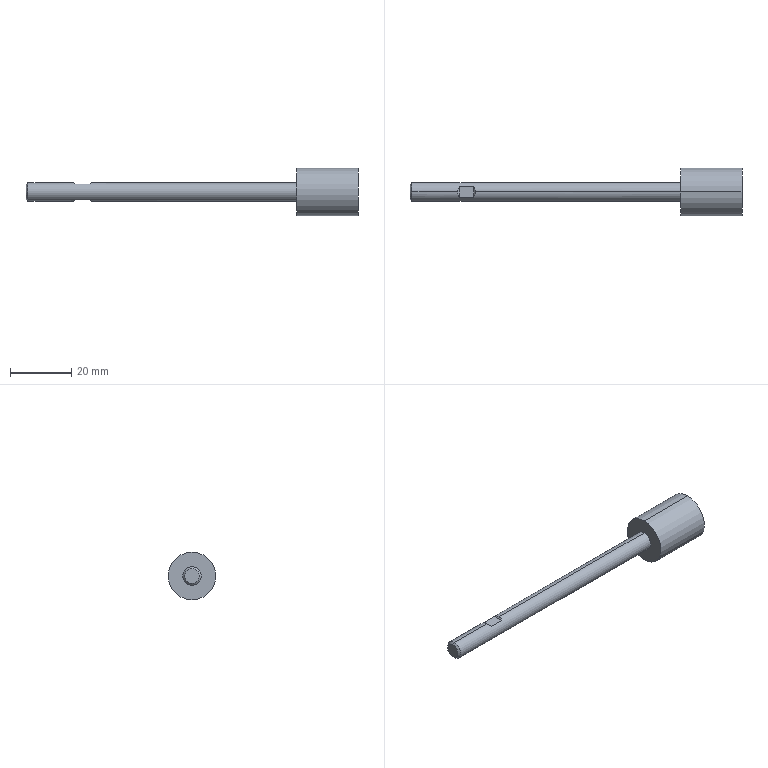Part | SolidWorks | features BaseBody 1 | 1 solid | 15 faces | box 108 x 15.5 x 15.5 mm | volume 6247 mm3 | plane 9 | cylinder 4 | cone 2 | commonest cylinder face diameters 6 x2 15.5 x2
STEP:
#1=CARTESIAN_POINT('',(88.,0.,3.));
#2=VERTEX_POINT('',#1);
#3=CARTESIAN_POINT('',(88.,0.,-3.));
#4=VERTEX_POINT('',#3);
#5=CARTESIAN_POINT('',(88.,0.,0.));
#6=DIRECTION('',(1.,0.,0.));
#7=DIRECTION('',(0.,0.,-1.));
#8=AXIS2_PLACEMENT_3D('',#5,#6,#7);
#9=CIRCLE('',#8,3.);
#10=EDGE_CURVE('',#2,#4,#9,.T.);
#11=ORIENTED_EDGE('',*,*,#10,.F.);
#12=CARTESIAN_POINT('',(21.3,0.,3.));
#13=VERTEX_POINT('',#12);
#14=CARTESIAN_POINT('',(108.,0.,3.));
#15=DIRECTION('',(-1.,0.,0.));
#16=VECTOR('',#15,1000.);
#17=LINE('',#14,#16);
#18=EDGE_CURVE('',#2,#13,#17,.T.);
#19=ORIENTED_EDGE('',*,*,#18,.T.);
#20=CARTESIAN_POINT('',(20.8,-1.658,2.5));
#21=VERTEX_POINT('',#20);
#22=CARTESIAN_POINT('',(20.8,-1.658,2.5));
#23=CARTESIAN_POINT('',(21.128,-1.163,2.828));
#24=CARTESIAN_POINT('',(21.3,-0.5942,3.));
#25=CARTESIAN_POINT('',(21.3,0.,3.));
#26=(BOUNDED_CURVE()B_SPLINE_CURVE(3,(#22,#23,#24,#25),.UNSPECIFIED.,.F.,.F.)B_SPLINE_CURVE_WITH_KNOTS((4,4),(5.697,6.283),.UNSPECIFIED.)CURVE()GEOMETRIC_REPRESENTATION_ITEM()RATIONAL_B_SPLINE_CURVE((1.,0.9716,0.9716,1.))REPRESENTATION_ITEM(''));
#27=EDGE_CURVE('',#21,#13,#26,.T.);
#28=ORIENTED_EDGE('',*,*,#27,.F.);
#29=CARTESIAN_POINT('',(16.,-1.658,2.5));
#30=VERTEX_POINT('',#29);
#31=CARTESIAN_POINT('',(108.,-1.658,2.5));
#32=DIRECTION('',(1.,0.,0.));
#33=VECTOR('',#32,1000.);
#34=LINE('',#31,#33);
#35=EDGE_CURVE('',#30,#21,#34,.T.);
#36=ORIENTED_EDGE('',*,*,#35,.F.);
#37=CARTESIAN_POINT('',(15.5,0.,3.));
#38=VERTEX_POINT('',#37);
#39=CARTESIAN_POINT('',(15.5,0.,3.));
#40=CARTESIAN_POINT('',(15.5,-0.5942,3.));
#41=CARTESIAN_POINT('',(15.672,-1.163,2.828));
#42=CARTESIAN_POINT('',(16.,-1.658,2.5));
#43=(BOUNDED_CURVE()B_SPLINE_CURVE(3,(#39,#40,#41,#42),.UNSPECIFIED.,.F.,.F.)B_SPLINE_CURVE_WITH_KNOTS((4,4),(3.142,3.727),.UNSPECIFIED.)CURVE()GEOMETRIC_REPRESENTATION_ITEM()RATIONAL_B_SPLINE_CURVE((1.,0.9716,0.9716,1.))REPRESENTATION_ITEM(''));
#44=EDGE_CURVE('',#38,#30,#43,.T.);
#45=ORIENTED_EDGE('',*,*,#44,.F.);
#46=CARTESIAN_POINT('',(0.6135,0.,3.));
#47=VERTEX_POINT('',#46);
#48=CARTESIAN_POINT('',(108.,0.,3.));
#49=DIRECTION('',(-1.,0.,0.));
#50=VECTOR('',#49,1000.);
#51=LINE('',#48,#50);
#52=EDGE_CURVE('',#38,#47,#51,.T.);
#53=ORIENTED_EDGE('',*,*,#52,.T.);
#54=CARTESIAN_POINT('',(0.6135,0.,-3.));
#55=VERTEX_POINT('',#54);
#56=CARTESIAN_POINT('',(0.6135,0.,0.));
#57=DIRECTION('',(1.,0.,0.));
#58=DIRECTION('',(0.,0.,-1.));
#59=AXIS2_PLACEMENT_3D('',#56,#57,#58);
#60=CIRCLE('',#59,3.);
#61=EDGE_CURVE('',#47,#55,#60,.T.);
#62=ORIENTED_EDGE('',*,*,#61,.T.);
#63=CARTESIAN_POINT('',(15.5,0.,-3.));
#64=VERTEX_POINT('',#63);
#65=CARTESIAN_POINT('',(108.,0.,-3.));
#66=DIRECTION('',(-1.,0.,0.));
#67=VECTOR('',#66,1000.);
#68=LINE('',#65,#67);
#69=EDGE_CURVE('',#64,#55,#68,.T.);
#70=ORIENTED_EDGE('',*,*,#69,.F.);
#71=CARTESIAN_POINT('',(16.,-1.658,-2.5));
#72=VERTEX_POINT('',#71);
#73=CARTESIAN_POINT('',(16.,-1.658,-2.5));
#74=CARTESIAN_POINT('',(15.672,-1.163,-2.828));
#75=CARTESIAN_POINT('',(15.5,-0.5942,-3.));
#76=CARTESIAN_POINT('',(15.5,0.,-3.));
#77=(BOUNDED_CURVE()B_SPLINE_CURVE(3,(#73,#74,#75,#76),.UNSPECIFIED.,.F.,.F.)B_SPLINE_CURVE_WITH_KNOTS((4,4),(2.556,3.142),.UNSPECIFIED.)CURVE()GEOMETRIC_REPRESENTATION_ITEM()RATIONAL_B_SPLINE_CURVE((1.,0.9716,0.9716,1.))REPRESENTATION_ITEM(''));
#78=EDGE_CURVE('',#72,#64,#77,.T.);
#79=ORIENTED_EDGE('',*,*,#78,.F.);
#80=CARTESIAN_POINT('',(20.8,-1.658,-2.5));
#81=VERTEX_POINT('',#80);
#82=CARTESIAN_POINT('',(108.,-1.658,-2.5));
#83=DIRECTION('',(-1.,0.,0.));
#84=VECTOR('',#83,1000.);
#85=LINE('',#82,#84);
#86=EDGE_CURVE('',#81,#72,#85,.T.);
#87=ORIENTED_EDGE('',*,*,#86,.F.);
#88=CARTESIAN_POINT('',(21.3,0.,-3.));
#89=VERTEX_POINT('',#88);
#90=CARTESIAN_POINT('',(21.3,0.,-3.));
#91=CARTESIAN_POINT('',(21.3,-0.5942,-3.));
#92=CARTESIAN_POINT('',(21.128,-1.163,-2.828));
#93=CARTESIAN_POINT('',(20.8,-1.658,-2.5));
#94=(BOUNDED_CURVE()B_SPLINE_CURVE(3,(#90,#91,#92,#93),.UNSPECIFIED.,.F.,.T.)B_SPLINE_CURVE_WITH_KNOTS((4,4),(0.,0.5857),.UNSPECIFIED.)CURVE()GEOMETRIC_REPRESENTATION_ITEM()RATIONAL_B_SPLINE_CURVE((1.,0.9716,0.9716,1.))REPRESENTATION_ITEM(''));
#95=EDGE_CURVE('',#89,#81,#94,.T.);
#96=ORIENTED_EDGE('',*,*,#95,.F.);
#97=CARTESIAN_POINT('',(108.,0.,-3.));
#98=DIRECTION('',(-1.,0.,0.));
#99=VECTOR('',#98,1000.);
#100=LINE('',#97,#99);
#101=EDGE_CURVE('',#4,#89,#100,.T.);
#102=ORIENTED_EDGE('',*,*,#101,.F.);
#103=EDGE_LOOP('',(#11,#19,#28,#36,#45,#53,#62,#70,#79,#87,#96,#102));
#104=FACE_OUTER_BOUND('',#103,.T.);
#105=CARTESIAN_POINT('',(108.,0.,0.));
#106=DIRECTION('',(-1.,0.,0.));
#107=DIRECTION('',(0.,0.,-1.));
#108=AXIS2_PLACEMENT_3D('',#105,#106,#107);
#109=CYLINDRICAL_SURFACE('',#108,3.);
#110=ADVANCED_FACE('',(#104),#109,.T.);
#111=CARTESIAN_POINT('',(0.,0.,-2.387));
#112=VERTEX_POINT('',#111);
#113=CARTESIAN_POINT('',(0.,0.,2.387));
#114=VERTEX_POINT('',#113);
#115=CARTESIAN_POINT('',(0.,0.,0.));
#116=DIRECTION('',(1.,0.,0.));
#117=DIRECTION('',(0.,0.,-1.));
#118=AXIS2_PLACEMENT_3D('',#115,#116,#117);
#119=CIRCLE('',#118,2.387);
#120=EDGE_CURVE('',#112,#114,#119,.T.);
#121=ORIENTED_EDGE('',*,*,#120,.T.);
#122=CARTESIAN_POINT('',(0.,0.,2.387));
#123=DIRECTION('',(0.7071,0.,0.7071));
#124=VECTOR('',#123,1000.);
#125=LINE('',#122,#124);
#126=EDGE_CURVE('',#114,#47,#125,.T.);
#127=ORIENTED_EDGE('',*,*,#126,.T.);
#128=CARTESIAN_POINT('',(0.6135,0.,0.));
#129=DIRECTION('',(1.,0.,0.));
#130=DIRECTION('',(0.,0.,-1.));
#131=AXIS2_PLACEMENT_3D('',#128,#129,#130);
#132=CIRCLE('',#131,3.);
#133=EDGE_CURVE('',#55,#47,#132,.T.);
#134=ORIENTED_EDGE('',*,*,#133,.F.);
#135=CARTESIAN_POINT('',(0.,0.,-2.387));
#136=DIRECTION('',(0.7071,0.,-0.7071));
#137=VECTOR('',#136,1000.);
#138=LINE('',#135,#137);
#139=EDGE_CURVE('',#112,#55,#138,.T.);
#140=ORIENTED_EDGE('',*,*,#139,.F.);
#141=EDGE_LOOP('',(#121,#127,#134,#140));
#142=FACE_OUTER_BOUND('',#141,.T.);
#143=CARTESIAN_POINT('',(0.,0.,0.));
#144=DIRECTION('',(1.,0.,0.));
#145=DIRECTION('',(0.,0.,-1.));
#146=AXIS2_PLACEMENT_3D('',#143,#144,#145);
#147=CONICAL_SURFACE('',#146,2.387,0.7854);
#148=ADVANCED_FACE('',(#142),#147,.T.);
#149=CARTESIAN_POINT('',(108.,0.,7.75));
#150=VERTEX_POINT('',#149);
#151=CARTESIAN_POINT('',(108.,0.,-7.75));
#152=VERTEX_POINT('',#151);
#153=CARTESIAN_POINT('',(108.,0.,0.));
#154=DIRECTION('',(1.,0.,0.));
#155=DIRECTION('',(0.,0.,-1.));
#156=AXIS2_PLACEMENT_3D('',#153,#154,#155);
#157=CIRCLE('',#156,7.75);
#158=EDGE_CURVE('',#150,#152,#157,.T.);
#159=ORIENTED_EDGE('',*,*,#158,.F.);
#160=CARTESIAN_POINT('',(88.,0.,7.75));
#161=VERTEX_POINT('',#160);
#162=CARTESIAN_POINT('',(108.,0.,7.75));
#163=DIRECTION('',(-1.,0.,0.));
#164=VECTOR('',#163,1000.);
#165=LINE('',#162,#164);
#166=EDGE_CURVE('',#150,#161,#165,.T.);
#167=ORIENTED_EDGE('',*,*,#166,.T.);
#168=CARTESIAN_POINT('',(88.,0.,-7.75));
#169=VERTEX_POINT('',#168);
#170=CARTESIAN_POINT('',(88.,0.,0.));
#171=DIRECTION('',(1.,0.,0.));
#172=DIRECTION('',(0.,0.,-1.));
#173=AXIS2_PLACEMENT_3D('',#170,#171,#172);
#174=CIRCLE('',#173,7.75);
#175=EDGE_CURVE('',#161,#169,#174,.T.);
#176=ORIENTED_EDGE('',*,*,#175,.T.);
#177=CARTESIAN_POINT('',(108.,0.,-7.75));
#178=DIRECTION('',(-1.,0.,0.));
#179=VECTOR('',#178,1000.);
#180=LINE('',#177,#179);
#181=EDGE_CURVE('',#152,#169,#180,.T.);
#182=ORIENTED_EDGE('',*,*,#181,.F.);
#183=EDGE_LOOP('',(#159,#167,#176,#182));
#184=FACE_OUTER_BOUND('',#183,.T.);
#185=CARTESIAN_POINT('',(108.,0.,0.));
#186=DIRECTION('',(-1.,0.,0.));
#187=DIRECTION('',(0.,0.,-1.));
#188=AXIS2_PLACEMENT_3D('',#185,#186,#187);
#189=CYLINDRICAL_SURFACE('',#188,7.75);
#190=ADVANCED_FACE('',(#184),#189,.T.);
#191=ORIENTED_EDGE('',*,*,#166,.F.);
#192=CARTESIAN_POINT('',(108.,0.,0.));
#193=DIRECTION('',(1.,0.,0.));
#194=DIRECTION('',(0.,0.,-1.));
#195=AXIS2_PLACEMENT_3D('',#192,#193,#194);
#196=CIRCLE('',#195,7.75);
#197=EDGE_CURVE('',#152,#150,#196,.T.);
#198=ORIENTED_EDGE('',*,*,#197,.F.);
#199=ORIENTED_EDGE('',*,*,#181,.T.);
#200=CARTESIAN_POINT('',(88.,0.,0.));
#201=DIRECTION('',(1.,0.,0.));
#202=DIRECTION('',(0.,0.,-1.));
#203=AXIS2_PLACEMENT_3D('',#200,#201,#202);
#204=CIRCLE('',#203,7.75);
#205=EDGE_CURVE('',#169,#161,#204,.T.);
#206=ORIENTED_EDGE('',*,*,#205,.T.);
#207=EDGE_LOOP('',(#191,#198,#199,#206));
#208=FACE_OUTER_BOUND('',#207,.T.);
#209=CARTESIAN_POINT('',(108.,0.,0.));
#210=DIRECTION('',(-1.,0.,0.));
#211=DIRECTION('',(0.,0.,-1.));
#212=AXIS2_PLACEMENT_3D('',#209,#210,#211);
#213=CYLINDRICAL_SURFACE('',#212,7.75);
#214=ADVANCED_FACE('',(#208),#213,.T.);
#215=ORIENTED_EDGE('',*,*,#197,.T.);
#216=ORIENTED_EDGE('',*,*,#158,.T.);
#217=EDGE_LOOP('',(#215,#216));
#218=FACE_OUTER_BOUND('',#217,.T.);
#219=CARTESIAN_POINT('',(108.,7.75,0.));
#220=DIRECTION('',(-1.,0.,0.));
#221=DIRECTION('',(0.,0.,1.));
#222=AXIS2_PLACEMENT_3D('',#219,#220,#221);
#223=PLANE('',#222);
#224=ADVANCED_FACE('',(#218),#223,.F.);
#225=CARTESIAN_POINT('',(20.8,1.658,-2.5));
#226=VERTEX_POINT('',#225);
#227=CARTESIAN_POINT('',(20.8,1.658,-2.5));
#228=CARTESIAN_POINT('',(21.128,1.163,-2.828));
#229=CARTESIAN_POINT('',(21.3,0.5942,-3.));
#230=CARTESIAN_POINT('',(21.3,0.,-3.));
#231=(BOUNDED_CURVE()B_SPLINE_CURVE(3,(#227,#228,#229,#230),.UNSPECIFIED.,.F.,.F.)B_SPLINE_CURVE_WITH_KNOTS((4,4),(5.697,6.283),.UNSPECIFIED.)CURVE()GEOMETRIC_REPRESENTATION_ITEM()RATIONAL_B_SPLINE_CURVE((1.,0.9716,0.9716,1.))REPRESENTATION_ITEM(''));
#232=EDGE_CURVE('',#226,#89,#231,.T.);
#233=ORIENTED_EDGE('',*,*,#232,.T.);
#234=ORIENTED_EDGE('',*,*,#95,.T.);
#235=CARTESIAN_POINT('',(20.8,2.5,-2.5));
#236=DIRECTION('',(0.,-1.,0.));
#237=VECTOR('',#236,1000.);
#238=LINE('',#235,#237);
#239=EDGE_CURVE('',#226,#81,#238,.T.);
#240=ORIENTED_EDGE('',*,*,#239,.F.);
#241=EDGE_LOOP('',(#233,#234,#240));
#242=FACE_OUTER_BOUND('',#241,.T.);
#243=CARTESIAN_POINT('',(20.8,2.5,-2.5));
#244=DIRECTION('',(-0.7071,0.,-0.7071));
#245=DIRECTION('',(-0.7071,0.,0.7071));
#246=AXIS2_PLACEMENT_3D('',#243,#244,#245);
#247=PLANE('',#246);
#248=ADVANCED_FACE('',(#242),#247,.T.);
#249=CARTESIAN_POINT('',(16.,1.658,-2.5));
#250=VERTEX_POINT('',#249);
#251=CARTESIAN_POINT('',(108.,1.658,-2.5));
#252=DIRECTION('',(1.,0.,0.));
#253=VECTOR('',#252,1000.);
#254=LINE('',#251,#253);
#255=EDGE_CURVE('',#250,#226,#254,.T.);
#256=ORIENTED_EDGE('',*,*,#255,.T.);
#257=ORIENTED_EDGE('',*,*,#239,.T.);
#258=ORIENTED_EDGE('',*,*,#86,.T.);
#259=CARTESIAN_POINT('',(16.,2.5,-2.5));
#260=DIRECTION('',(0.,-1.,0.));
#261=VECTOR('',#260,1000.);
#262=LINE('',#259,#261);
#263=EDGE_CURVE('',#250,#72,#262,.T.);
#264=ORIENTED_EDGE('',*,*,#263,.F.);
#265=EDGE_LOOP('',(#256,#257,#258,#264));
#266=FACE_OUTER_BOUND('',#265,.T.);
#267=CARTESIAN_POINT('',(16.,2.5,-2.5));
#268=DIRECTION('',(0.,0.,-1.));
#269=DIRECTION('',(0.,-1.,0.));
#270=AXIS2_PLACEMENT_3D('',#267,#268,#269);
#271=PLANE('',#270);
#272=ADVANCED_FACE('',(#266),#271,.T.);
#273=ORIENTED_EDGE('',*,*,#27,.T.);
#274=CARTESIAN_POINT('',(20.8,1.658,2.5));
#275=VERTEX_POINT('',#274);
#276=CARTESIAN_POINT('',(21.3,0.,3.));
#277=CARTESIAN_POINT('',(21.3,0.5942,3.));
#278=CARTESIAN_POINT('',(21.128,1.163,2.828));
#279=CARTESIAN_POINT('',(20.8,1.658,2.5));
#280=(BOUNDED_CURVE()B_SPLINE_CURVE(3,(#276,#277,#278,#279),.UNSPECIFIED.,.F.,.F.)B_SPLINE_CURVE_WITH_KNOTS((4,4),(0.,0.5857),.UNSPECIFIED.)CURVE()GEOMETRIC_REPRESENTATION_ITEM()RATIONAL_B_SPLINE_CURVE((1.,0.9716,0.9716,1.))REPRESENTATION_ITEM(''));
#281=EDGE_CURVE('',#13,#275,#280,.T.);
#282=ORIENTED_EDGE('',*,*,#281,.T.);
#283=CARTESIAN_POINT('',(20.8,2.5,2.5));
#284=DIRECTION('',(0.,-1.,0.));
#285=VECTOR('',#284,1000.);
#286=LINE('',#283,#285);
#287=EDGE_CURVE('',#275,#21,#286,.T.);
#288=ORIENTED_EDGE('',*,*,#287,.T.);
#289=EDGE_LOOP('',(#273,#282,#288));
#290=FACE_OUTER_BOUND('',#289,.T.);
#291=CARTESIAN_POINT('',(30.3,2.5,12.));
#292=DIRECTION('',(-0.7071,0.,0.7071));
#293=DIRECTION('',(0.,1.,0.));
#294=AXIS2_PLACEMENT_3D('',#291,#292,#293);
#295=PLANE('',#294);
#296=ADVANCED_FACE('',(#290),#295,.T.);
#297=ORIENTED_EDGE('',*,*,#78,.T.);
#298=CARTESIAN_POINT('',(15.5,0.,-3.));
#299=CARTESIAN_POINT('',(15.5,0.5942,-3.));
#300=CARTESIAN_POINT('',(15.672,1.163,-2.828));
#301=CARTESIAN_POINT('',(16.,1.658,-2.5));
#302=(BOUNDED_CURVE()B_SPLINE_CURVE(3,(#298,#299,#300,#301),.UNSPECIFIED.,.F.,.F.)B_SPLINE_CURVE_WITH_KNOTS((4,4),(3.142,3.727),.UNSPECIFIED.)CURVE()GEOMETRIC_REPRESENTATION_ITEM()RATIONAL_B_SPLINE_CURVE((1.,0.9716,0.9716,1.))REPRESENTATION_ITEM(''));
#303=EDGE_CURVE('',#64,#250,#302,.T.);
#304=ORIENTED_EDGE('',*,*,#303,.T.);
#305=ORIENTED_EDGE('',*,*,#263,.T.);
#306=EDGE_LOOP('',(#297,#304,#305));
#307=FACE_OUTER_BOUND('',#306,.T.);
#308=CARTESIAN_POINT('',(14.4,2.5,-4.1));
#309=DIRECTION('',(0.7071,0.,-0.7071));
#310=DIRECTION('',(0.,-1.,0.));
#311=AXIS2_PLACEMENT_3D('',#308,#309,#310);
#312=PLANE('',#311);
#313=ADVANCED_FACE('',(#307),#312,.T.);
#314=CARTESIAN_POINT('',(88.,0.,0.));
#315=DIRECTION('',(1.,0.,0.));
#316=DIRECTION('',(0.,0.,-1.));
#317=AXIS2_PLACEMENT_3D('',#314,#315,#316);
#318=CIRCLE('',#317,3.);
#319=EDGE_CURVE('',#4,#2,#318,.T.);
#320=ORIENTED_EDGE('',*,*,#319,.T.);
#321=ORIENTED_EDGE('',*,*,#10,.T.);
#322=EDGE_LOOP('',(#320,#321));
#323=FACE_BOUND('',#322,.T.);
#324=ORIENTED_EDGE('',*,*,#205,.F.);
#325=ORIENTED_EDGE('',*,*,#175,.F.);
#326=EDGE_LOOP('',(#324,#325));
#327=FACE_OUTER_BOUND('',#326,.T.);
#328=CARTESIAN_POINT('',(88.,3.,0.));
#329=DIRECTION('',(1.,0.,0.));
#330=DIRECTION('',(0.,1.,0.));
#331=AXIS2_PLACEMENT_3D('',#328,#329,#330);
#332=PLANE('',#331);
#333=ADVANCED_FACE('',(#323,#327),#332,.F.);
#334=ORIENTED_EDGE('',*,*,#126,.F.);
#335=CARTESIAN_POINT('',(0.,0.,0.));
#336=DIRECTION('',(1.,0.,0.));
#337=DIRECTION('',(0.,0.,-1.));
#338=AXIS2_PLACEMENT_3D('',#335,#336,#337);
#339=CIRCLE('',#338,2.387);
#340=EDGE_CURVE('',#114,#112,#339,.T.);
#341=ORIENTED_EDGE('',*,*,#340,.T.);
#342=ORIENTED_EDGE('',*,*,#139,.T.);
#343=ORIENTED_EDGE('',*,*,#61,.F.);
#344=EDGE_LOOP('',(#334,#341,#342,#343));
#345=FACE_OUTER_BOUND('',#344,.T.);
#346=CARTESIAN_POINT('',(0.,0.,0.));
#347=DIRECTION('',(1.,0.,0.));
#348=DIRECTION('',(0.,0.,-1.));
#349=AXIS2_PLACEMENT_3D('',#346,#347,#348);
#350=CONICAL_SURFACE('',#349,2.387,0.7854);
#351=ADVANCED_FACE('',(#345),#350,.T.);
#352=ORIENTED_EDGE('',*,*,#120,.F.);
#353=ORIENTED_EDGE('',*,*,#340,.F.);
#354=EDGE_LOOP('',(#352,#353));
#355=FACE_OUTER_BOUND('',#354,.T.);
#356=CARTESIAN_POINT('',(0.,0.,0.));
#357=DIRECTION('',(1.,0.,0.));
#358=DIRECTION('',(0.,1.,0.));
#359=AXIS2_PLACEMENT_3D('',#356,#357,#358);
#360=PLANE('',#359);
#361=ADVANCED_FACE('',(#355),#360,.F.);
#362=ORIENTED_EDGE('',*,*,#18,.F.);
#363=ORIENTED_EDGE('',*,*,#319,.F.);
#364=ORIENTED_EDGE('',*,*,#101,.T.);
#365=ORIENTED_EDGE('',*,*,#232,.F.);
#366=ORIENTED_EDGE('',*,*,#255,.F.);
#367=ORIENTED_EDGE('',*,*,#303,.F.);
#368=ORIENTED_EDGE('',*,*,#69,.T.);
#369=ORIENTED_EDGE('',*,*,#133,.T.);
#370=ORIENTED_EDGE('',*,*,#52,.F.);
#371=CARTESIAN_POINT('',(16.,1.658,2.5));
#372=VERTEX_POINT('',#371);
#373=CARTESIAN_POINT('',(16.,1.658,2.5));
#374=CARTESIAN_POINT('',(15.672,1.163,2.828));
#375=CARTESIAN_POINT('',(15.5,0.5942,3.));
#376=CARTESIAN_POINT('',(15.5,0.,3.));
#377=(BOUNDED_CURVE()B_SPLINE_CURVE(3,(#373,#374,#375,#376),.UNSPECIFIED.,.F.,.F.)B_SPLINE_CURVE_WITH_KNOTS((4,4),(2.556,3.142),.UNSPECIFIED.)CURVE()GEOMETRIC_REPRESENTATION_ITEM()RATIONAL_B_SPLINE_CURVE((1.,0.9716,0.9716,1.))REPRESENTATION_ITEM(''));
#378=EDGE_CURVE('',#372,#38,#377,.T.);
#379=ORIENTED_EDGE('',*,*,#378,.F.);
#380=CARTESIAN_POINT('',(108.,1.658,2.5));
#381=DIRECTION('',(-1.,0.,0.));
#382=VECTOR('',#381,1000.);
#383=LINE('',#380,#382);
#384=EDGE_CURVE('',#275,#372,#383,.T.);
#385=ORIENTED_EDGE('',*,*,#384,.F.);
#386=ORIENTED_EDGE('',*,*,#281,.F.);
#387=EDGE_LOOP('',(#362,#363,#364,#365,#366,#367,#368,#369,#370,#379,#385,#386));
#388=FACE_OUTER_BOUND('',#387,.T.);
#389=CARTESIAN_POINT('',(108.,0.,0.));
#390=DIRECTION('',(-1.,0.,0.));
#391=DIRECTION('',(0.,0.,-1.));
#392=AXIS2_PLACEMENT_3D('',#389,#390,#391);
#393=CYLINDRICAL_SURFACE('',#392,3.);
#394=ADVANCED_FACE('',(#388),#393,.T.);
#395=ORIENTED_EDGE('',*,*,#35,.T.);
#396=ORIENTED_EDGE('',*,*,#287,.F.);
#397=ORIENTED_EDGE('',*,*,#384,.T.);
#398=CARTESIAN_POINT('',(16.,2.5,2.5));
#399=DIRECTION('',(0.,-1.,0.));
#400=VECTOR('',#399,1000.);
#401=LINE('',#398,#400);
#402=EDGE_CURVE('',#372,#30,#401,.T.);
#403=ORIENTED_EDGE('',*,*,#402,.T.);
#404=EDGE_LOOP('',(#395,#396,#397,#403));
#405=FACE_OUTER_BOUND('',#404,.T.);
#406=CARTESIAN_POINT('',(20.8,2.5,2.5));
#407=DIRECTION('',(0.,0.,1.));
#408=DIRECTION('',(1.,0.,0.));
#409=AXIS2_PLACEMENT_3D('',#406,#407,#408);
#410=PLANE('',#409);
#411=ADVANCED_FACE('',(#405),#410,.T.);
#412=ORIENTED_EDGE('',*,*,#378,.T.);
#413=ORIENTED_EDGE('',*,*,#44,.T.);
#414=ORIENTED_EDGE('',*,*,#402,.F.);
#415=EDGE_LOOP('',(#412,#413,#414));
#416=FACE_OUTER_BOUND('',#415,.T.);
#417=CARTESIAN_POINT('',(16.,2.5,2.5));
#418=DIRECTION('',(0.7071,0.,0.7071));
#419=DIRECTION('',(0.,-1.,0.));
#420=AXIS2_PLACEMENT_3D('',#417,#418,#419);
#421=PLANE('',#420);
#422=ADVANCED_FACE('',(#416),#421,.T.);
#423=CLOSED_SHELL('',(#110,#148,#190,#214,#224,#248,#272,#296,#313,#333,#351,#361,#394,#411,#422));
#424=MANIFOLD_SOLID_BREP('',#423);
#425=CARTESIAN_POINT('',(0.,0.,0.));
#426=DIRECTION('',(0.,0.,1.));
#427=DIRECTION('',(1.,0.,0.));
#428=AXIS2_PLACEMENT_3D('',#425,#426,#427);
#429=(LENGTH_UNIT()NAMED_UNIT(*)SI_UNIT(.MILLI.,.METRE.));
#430=UNCERTAINTY_MEASURE_WITH_UNIT(LENGTH_MEASURE(0.00001),#429,'','');
#431=(NAMED_UNIT(*)PLANE_ANGLE_UNIT()SI_UNIT($,.RADIAN.));
#432=(NAMED_UNIT(*)SI_UNIT($,.STERADIAN.)SOLID_ANGLE_UNIT());
#433=(GEOMETRIC_REPRESENTATION_CONTEXT(3)GLOBAL_UNCERTAINTY_ASSIGNED_CONTEXT((#430))GLOBAL_UNIT_ASSIGNED_CONTEXT((#429,#431,#432))REPRESENTATION_CONTEXT('',''));
#434=ADVANCED_BREP_SHAPE_REPRESENTATION('',(#424,#428),#433);